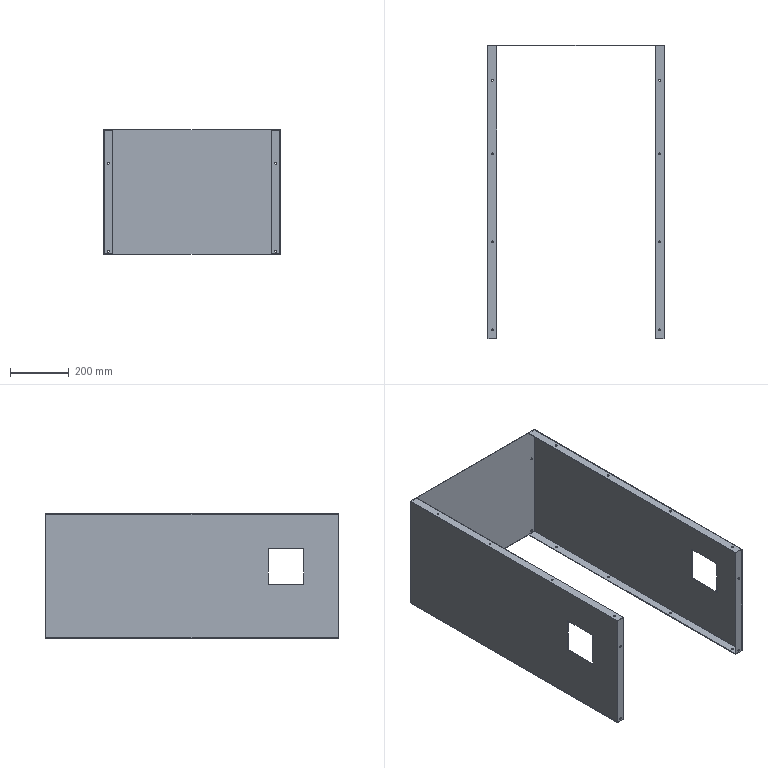Part | SolidWorks | features ICE 5, Extrusion 1, Shell 1 | 1 solid | 74 faces | box 600 x 1000 x 425 mm | volume 2418347 mm3 | cylinder 48 | plane 26 | commonest cylinder face diameters 6 x48